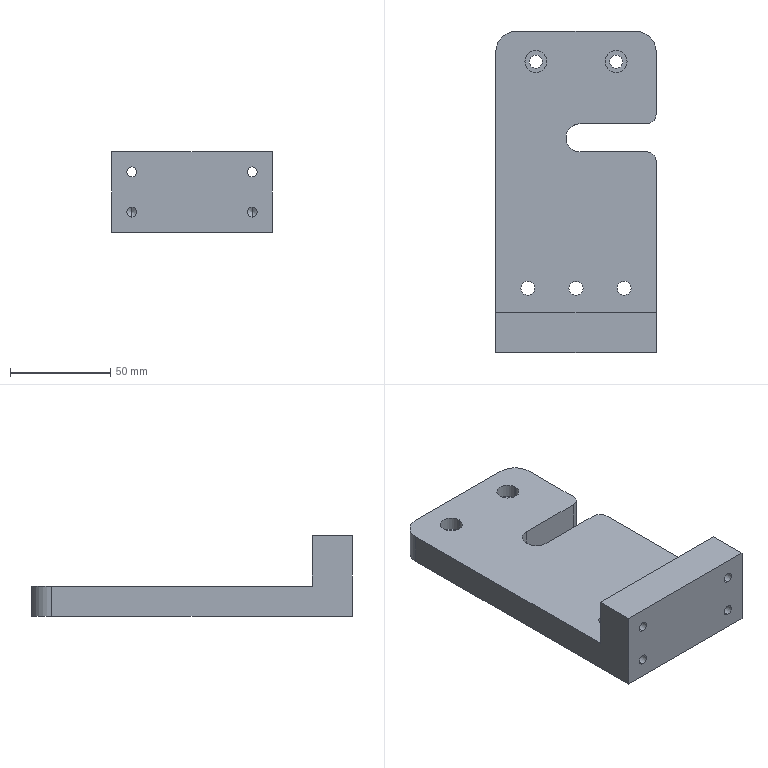Part | SolidWorks | features BaseBody 1 | 1 solid | 44 faces | box 80 x 160 x 40 mm | volume 216767 mm3 | cylinder 27 | plane 13 | cone 4 | commonest cylinder face diameters 5 x8 7 x6 6.6 x4 11 x4 10 x2 20 x2
STEP:
#1=CARTESIAN_POINT('',(-25.5,65.,8.2));
#2=VERTEX_POINT('',#1);
#3=CARTESIAN_POINT('',(-14.5,65.,8.2));
#4=VERTEX_POINT('',#3);
#5=CARTESIAN_POINT('',(-20.,65.,8.2));
#6=DIRECTION('',(0.,0.,1.));
#7=DIRECTION('',(1.,0.,0.));
#8=AXIS2_PLACEMENT_3D('',#5,#6,#7);
#9=CIRCLE('',#8,5.5);
#10=EDGE_CURVE('',#2,#4,#9,.T.);
#11=ORIENTED_EDGE('',*,*,#10,.F.);
#12=CARTESIAN_POINT('',(-25.5,65.,15.));
#13=VERTEX_POINT('',#12);
#14=CARTESIAN_POINT('',(-25.5,65.,15.));
#15=DIRECTION('',(0.,0.,1.));
#16=VECTOR('',#15,1000.);
#17=LINE('',#14,#16);
#18=EDGE_CURVE('',#2,#13,#17,.T.);
#19=ORIENTED_EDGE('',*,*,#18,.T.);
#20=CARTESIAN_POINT('',(-14.5,65.,15.));
#21=VERTEX_POINT('',#20);
#22=CARTESIAN_POINT('',(-20.,65.,15.));
#23=DIRECTION('',(0.,0.,1.));
#24=DIRECTION('',(1.,0.,0.));
#25=AXIS2_PLACEMENT_3D('',#22,#23,#24);
#26=CIRCLE('',#25,5.5);
#27=EDGE_CURVE('',#13,#21,#26,.T.);
#28=ORIENTED_EDGE('',*,*,#27,.T.);
#29=CARTESIAN_POINT('',(-14.5,65.,15.));
#30=DIRECTION('',(0.,0.,1.));
#31=VECTOR('',#30,1000.);
#32=LINE('',#29,#31);
#33=EDGE_CURVE('',#4,#21,#32,.T.);
#34=ORIENTED_EDGE('',*,*,#33,.F.);
#35=EDGE_LOOP('',(#11,#19,#28,#34));
#36=FACE_OUTER_BOUND('',#35,.T.);
#37=CARTESIAN_POINT('',(-20.,65.,15.));
#38=DIRECTION('',(0.,0.,1.));
#39=DIRECTION('',(1.,0.,0.));
#40=AXIS2_PLACEMENT_3D('',#37,#38,#39);
#41=CYLINDRICAL_SURFACE('',#40,5.5);
#42=ADVANCED_FACE('',(#36),#41,.F.);
#43=CARTESIAN_POINT('',(-23.3,65.,0.));
#44=VERTEX_POINT('',#43);
#45=CARTESIAN_POINT('',(-16.7,65.,0.));
#46=VERTEX_POINT('',#45);
#47=CARTESIAN_POINT('',(-20.,65.,0.));
#48=DIRECTION('',(0.,0.,1.));
#49=DIRECTION('',(1.,0.,0.));
#50=AXIS2_PLACEMENT_3D('',#47,#48,#49);
#51=CIRCLE('',#50,3.3);
#52=EDGE_CURVE('',#44,#46,#51,.T.);
#53=ORIENTED_EDGE('',*,*,#52,.F.);
#54=CARTESIAN_POINT('',(-23.3,65.,8.2));
#55=VERTEX_POINT('',#54);
#56=CARTESIAN_POINT('',(-23.3,65.,15.));
#57=DIRECTION('',(0.,0.,1.));
#58=VECTOR('',#57,1000.);
#59=LINE('',#56,#58);
#60=EDGE_CURVE('',#44,#55,#59,.T.);
#61=ORIENTED_EDGE('',*,*,#60,.T.);
#62=CARTESIAN_POINT('',(-16.7,65.,8.2));
#63=VERTEX_POINT('',#62);
#64=CARTESIAN_POINT('',(-20.,65.,8.2));
#65=DIRECTION('',(0.,0.,1.));
#66=DIRECTION('',(1.,0.,0.));
#67=AXIS2_PLACEMENT_3D('',#64,#65,#66);
#68=CIRCLE('',#67,3.3);
#69=EDGE_CURVE('',#55,#63,#68,.T.);
#70=ORIENTED_EDGE('',*,*,#69,.T.);
#71=CARTESIAN_POINT('',(-16.7,65.,15.));
#72=DIRECTION('',(0.,0.,1.));
#73=VECTOR('',#72,1000.);
#74=LINE('',#71,#73);
#75=EDGE_CURVE('',#46,#63,#74,.T.);
#76=ORIENTED_EDGE('',*,*,#75,.F.);
#77=EDGE_LOOP('',(#53,#61,#70,#76));
#78=FACE_OUTER_BOUND('',#77,.T.);
#79=CARTESIAN_POINT('',(-20.,65.,15.));
#80=DIRECTION('',(0.,0.,1.));
#81=DIRECTION('',(1.,0.,0.));
#82=AXIS2_PLACEMENT_3D('',#79,#80,#81);
#83=CYLINDRICAL_SURFACE('',#82,3.3);
#84=ADVANCED_FACE('',(#78),#83,.F.);
#85=CARTESIAN_POINT('',(14.5,65.,8.2));
#86=VERTEX_POINT('',#85);
#87=CARTESIAN_POINT('',(25.5,65.,8.2));
#88=VERTEX_POINT('',#87);
#89=CARTESIAN_POINT('',(20.,65.,8.2));
#90=DIRECTION('',(0.,0.,1.));
#91=DIRECTION('',(1.,0.,0.));
#92=AXIS2_PLACEMENT_3D('',#89,#90,#91);
#93=CIRCLE('',#92,5.5);
#94=EDGE_CURVE('',#86,#88,#93,.T.);
#95=ORIENTED_EDGE('',*,*,#94,.F.);
#96=CARTESIAN_POINT('',(14.5,65.,15.));
#97=VERTEX_POINT('',#96);
#98=CARTESIAN_POINT('',(14.5,65.,15.));
#99=DIRECTION('',(0.,0.,1.));
#100=VECTOR('',#99,1000.);
#101=LINE('',#98,#100);
#102=EDGE_CURVE('',#86,#97,#101,.T.);
#103=ORIENTED_EDGE('',*,*,#102,.T.);
#104=CARTESIAN_POINT('',(25.5,65.,15.));
#105=VERTEX_POINT('',#104);
#106=CARTESIAN_POINT('',(20.,65.,15.));
#107=DIRECTION('',(0.,0.,1.));
#108=DIRECTION('',(1.,0.,0.));
#109=AXIS2_PLACEMENT_3D('',#106,#107,#108);
#110=CIRCLE('',#109,5.5);
#111=EDGE_CURVE('',#97,#105,#110,.T.);
#112=ORIENTED_EDGE('',*,*,#111,.T.);
#113=CARTESIAN_POINT('',(25.5,65.,15.));
#114=DIRECTION('',(0.,0.,1.));
#115=VECTOR('',#114,1000.);
#116=LINE('',#113,#115);
#117=EDGE_CURVE('',#88,#105,#116,.T.);
#118=ORIENTED_EDGE('',*,*,#117,.F.);
#119=EDGE_LOOP('',(#95,#103,#112,#118));
#120=FACE_OUTER_BOUND('',#119,.T.);
#121=CARTESIAN_POINT('',(20.,65.,15.));
#122=DIRECTION('',(0.,0.,1.));
#123=DIRECTION('',(1.,0.,0.));
#124=AXIS2_PLACEMENT_3D('',#121,#122,#123);
#125=CYLINDRICAL_SURFACE('',#124,5.5);
#126=ADVANCED_FACE('',(#120),#125,.F.);
#127=CARTESIAN_POINT('',(16.7,65.,0.));
#128=VERTEX_POINT('',#127);
#129=CARTESIAN_POINT('',(23.3,65.,0.));
#130=VERTEX_POINT('',#129);
#131=CARTESIAN_POINT('',(20.,65.,0.));
#132=DIRECTION('',(0.,0.,1.));
#133=DIRECTION('',(1.,0.,0.));
#134=AXIS2_PLACEMENT_3D('',#131,#132,#133);
#135=CIRCLE('',#134,3.3);
#136=EDGE_CURVE('',#128,#130,#135,.T.);
#137=ORIENTED_EDGE('',*,*,#136,.F.);
#138=CARTESIAN_POINT('',(16.7,65.,8.2));
#139=VERTEX_POINT('',#138);
#140=CARTESIAN_POINT('',(16.7,65.,15.));
#141=DIRECTION('',(0.,0.,1.));
#142=VECTOR('',#141,1000.);
#143=LINE('',#140,#142);
#144=EDGE_CURVE('',#128,#139,#143,.T.);
#145=ORIENTED_EDGE('',*,*,#144,.T.);
#146=CARTESIAN_POINT('',(23.3,65.,8.2));
#147=VERTEX_POINT('',#146);
#148=CARTESIAN_POINT('',(20.,65.,8.2));
#149=DIRECTION('',(0.,0.,1.));
#150=DIRECTION('',(1.,0.,0.));
#151=AXIS2_PLACEMENT_3D('',#148,#149,#150);
#152=CIRCLE('',#151,3.3);
#153=EDGE_CURVE('',#139,#147,#152,.T.);
#154=ORIENTED_EDGE('',*,*,#153,.T.);
#155=CARTESIAN_POINT('',(23.3,65.,15.));
#156=DIRECTION('',(0.,0.,1.));
#157=VECTOR('',#156,1000.);
#158=LINE('',#155,#157);
#159=EDGE_CURVE('',#130,#147,#158,.T.);
#160=ORIENTED_EDGE('',*,*,#159,.F.);
#161=EDGE_LOOP('',(#137,#145,#154,#160));
#162=FACE_OUTER_BOUND('',#161,.T.);
#163=CARTESIAN_POINT('',(20.,65.,15.));
#164=DIRECTION('',(0.,0.,1.));
#165=DIRECTION('',(1.,0.,0.));
#166=AXIS2_PLACEMENT_3D('',#163,#164,#165);
#167=CYLINDRICAL_SURFACE('',#166,3.3);
#168=ADVANCED_FACE('',(#162),#167,.F.);
#169=CARTESIAN_POINT('',(-27.5,-48.,0.));
#170=VERTEX_POINT('',#169);
#171=CARTESIAN_POINT('',(-20.5,-48.,0.));
#172=VERTEX_POINT('',#171);
#173=CARTESIAN_POINT('',(-24.,-48.,0.));
#174=DIRECTION('',(0.,0.,1.));
#175=DIRECTION('',(1.,0.,0.));
#176=AXIS2_PLACEMENT_3D('',#173,#174,#175);
#177=CIRCLE('',#176,3.5);
#178=EDGE_CURVE('',#170,#172,#177,.T.);
#179=ORIENTED_EDGE('',*,*,#178,.F.);
#180=CARTESIAN_POINT('',(-27.5,-48.,15.));
#181=VERTEX_POINT('',#180);
#182=CARTESIAN_POINT('',(-27.5,-48.,15.));
#183=DIRECTION('',(0.,0.,1.));
#184=VECTOR('',#183,1000.);
#185=LINE('',#182,#184);
#186=EDGE_CURVE('',#170,#181,#185,.T.);
#187=ORIENTED_EDGE('',*,*,#186,.T.);
#188=CARTESIAN_POINT('',(-20.5,-48.,15.));
#189=VERTEX_POINT('',#188);
#190=CARTESIAN_POINT('',(-24.,-48.,15.));
#191=DIRECTION('',(0.,0.,1.));
#192=DIRECTION('',(1.,0.,0.));
#193=AXIS2_PLACEMENT_3D('',#190,#191,#192);
#194=CIRCLE('',#193,3.5);
#195=EDGE_CURVE('',#181,#189,#194,.T.);
#196=ORIENTED_EDGE('',*,*,#195,.T.);
#197=CARTESIAN_POINT('',(-20.5,-48.,15.));
#198=DIRECTION('',(0.,0.,1.));
#199=VECTOR('',#198,1000.);
#200=LINE('',#197,#199);
#201=EDGE_CURVE('',#172,#189,#200,.T.);
#202=ORIENTED_EDGE('',*,*,#201,.F.);
#203=EDGE_LOOP('',(#179,#187,#196,#202));
#204=FACE_OUTER_BOUND('',#203,.T.);
#205=CARTESIAN_POINT('',(-24.,-48.,15.));
#206=DIRECTION('',(0.,0.,1.));
#207=DIRECTION('',(1.,0.,0.));
#208=AXIS2_PLACEMENT_3D('',#205,#206,#207);
#209=CYLINDRICAL_SURFACE('',#208,3.5);
#210=ADVANCED_FACE('',(#204),#209,.F.);
#211=CARTESIAN_POINT('',(-3.5,-48.,0.));
#212=VERTEX_POINT('',#211);
#213=CARTESIAN_POINT('',(3.5,-48.,0.));
#214=VERTEX_POINT('',#213);
#215=CARTESIAN_POINT('',(0.,-48.,0.));
#216=DIRECTION('',(0.,0.,1.));
#217=DIRECTION('',(1.,0.,0.));
#218=AXIS2_PLACEMENT_3D('',#215,#216,#217);
#219=CIRCLE('',#218,3.5);
#220=EDGE_CURVE('',#212,#214,#219,.T.);
#221=ORIENTED_EDGE('',*,*,#220,.F.);
#222=CARTESIAN_POINT('',(-3.5,-48.,15.));
#223=VERTEX_POINT('',#222);
#224=CARTESIAN_POINT('',(-3.5,-48.,15.));
#225=DIRECTION('',(0.,0.,1.));
#226=VECTOR('',#225,1000.);
#227=LINE('',#224,#226);
#228=EDGE_CURVE('',#212,#223,#227,.T.);
#229=ORIENTED_EDGE('',*,*,#228,.T.);
#230=CARTESIAN_POINT('',(3.5,-48.,15.));
#231=VERTEX_POINT('',#230);
#232=CARTESIAN_POINT('',(0.,-48.,15.));
#233=DIRECTION('',(0.,0.,1.));
#234=DIRECTION('',(1.,0.,0.));
#235=AXIS2_PLACEMENT_3D('',#232,#233,#234);
#236=CIRCLE('',#235,3.5);
#237=EDGE_CURVE('',#223,#231,#236,.T.);
#238=ORIENTED_EDGE('',*,*,#237,.T.);
#239=CARTESIAN_POINT('',(3.5,-48.,15.));
#240=DIRECTION('',(0.,0.,1.));
#241=VECTOR('',#240,1000.);
#242=LINE('',#239,#241);
#243=EDGE_CURVE('',#214,#231,#242,.T.);
#244=ORIENTED_EDGE('',*,*,#243,.F.);
#245=EDGE_LOOP('',(#221,#229,#238,#244));
#246=FACE_OUTER_BOUND('',#245,.T.);
#247=CARTESIAN_POINT('',(0.,-48.,15.));
#248=DIRECTION('',(0.,0.,1.));
#249=DIRECTION('',(1.,0.,0.));
#250=AXIS2_PLACEMENT_3D('',#247,#248,#249);
#251=CYLINDRICAL_SURFACE('',#250,3.5);
#252=ADVANCED_FACE('',(#246),#251,.F.);
#253=CARTESIAN_POINT('',(20.5,-48.,0.));
#254=VERTEX_POINT('',#253);
#255=CARTESIAN_POINT('',(27.5,-48.,0.));
#256=VERTEX_POINT('',#255);
#257=CARTESIAN_POINT('',(24.,-48.,0.));
#258=DIRECTION('',(0.,0.,1.));
#259=DIRECTION('',(1.,0.,0.));
#260=AXIS2_PLACEMENT_3D('',#257,#258,#259);
#261=CIRCLE('',#260,3.5);
#262=EDGE_CURVE('',#254,#256,#261,.T.);
#263=ORIENTED_EDGE('',*,*,#262,.F.);
#264=CARTESIAN_POINT('',(20.5,-48.,15.));
#265=VERTEX_POINT('',#264);
#266=CARTESIAN_POINT('',(20.5,-48.,15.));
#267=DIRECTION('',(0.,0.,1.));
#268=VECTOR('',#267,1000.);
#269=LINE('',#266,#268);
#270=EDGE_CURVE('',#254,#265,#269,.T.);
#271=ORIENTED_EDGE('',*,*,#270,.T.);
#272=CARTESIAN_POINT('',(27.5,-48.,15.));
#273=VERTEX_POINT('',#272);
#274=CARTESIAN_POINT('',(24.,-48.,15.));
#275=DIRECTION('',(0.,0.,1.));
#276=DIRECTION('',(1.,0.,0.));
#277=AXIS2_PLACEMENT_3D('',#274,#275,#276);
#278=CIRCLE('',#277,3.5);
#279=EDGE_CURVE('',#265,#273,#278,.T.);
#280=ORIENTED_EDGE('',*,*,#279,.T.);
#281=CARTESIAN_POINT('',(27.5,-48.,15.));
#282=DIRECTION('',(0.,0.,1.));
#283=VECTOR('',#282,1000.);
#284=LINE('',#281,#283);
#285=EDGE_CURVE('',#256,#273,#284,.T.);
#286=ORIENTED_EDGE('',*,*,#285,.F.);
#287=EDGE_LOOP('',(#263,#271,#280,#286));
#288=FACE_OUTER_BOUND('',#287,.T.);
#289=CARTESIAN_POINT('',(24.,-48.,15.));
#290=DIRECTION('',(0.,0.,1.));
#291=DIRECTION('',(1.,0.,0.));
#292=AXIS2_PLACEMENT_3D('',#289,#290,#291);
#293=CYLINDRICAL_SURFACE('',#292,3.5);
#294=ADVANCED_FACE('',(#288),#293,.F.);
#295=CARTESIAN_POINT('',(30.,-60.,32.5));
#296=VERTEX_POINT('',#295);
#297=CARTESIAN_POINT('',(30.,-60.,27.5));
#298=VERTEX_POINT('',#297);
#299=CARTESIAN_POINT('',(30.,-60.,30.));
#300=DIRECTION('',(0.,-1.,0.));
#301=DIRECTION('',(0.,0.,-1.));
#302=AXIS2_PLACEMENT_3D('',#299,#300,#301);
#303=CIRCLE('',#302,2.5);
#304=EDGE_CURVE('',#296,#298,#303,.T.);
#305=ORIENTED_EDGE('',*,*,#304,.F.);
#306=CARTESIAN_POINT('',(30.,-80.,32.5));
#307=VERTEX_POINT('',#306);
#308=CARTESIAN_POINT('',(30.,-80.,32.5));
#309=DIRECTION('',(0.,-1.,0.));
#310=VECTOR('',#309,1000.);
#311=LINE('',#308,#310);
#312=EDGE_CURVE('',#296,#307,#311,.T.);
#313=ORIENTED_EDGE('',*,*,#312,.T.);
#314=CARTESIAN_POINT('',(30.,-80.,27.5));
#315=VERTEX_POINT('',#314);
#316=CARTESIAN_POINT('',(30.,-80.,30.));
#317=DIRECTION('',(0.,-1.,0.));
#318=DIRECTION('',(0.,0.,-1.));
#319=AXIS2_PLACEMENT_3D('',#316,#317,#318);
#320=CIRCLE('',#319,2.5);
#321=EDGE_CURVE('',#307,#315,#320,.T.);
#322=ORIENTED_EDGE('',*,*,#321,.T.);
#323=CARTESIAN_POINT('',(30.,-80.,27.5));
#324=DIRECTION('',(0.,-1.,0.));
#325=VECTOR('',#324,1000.);
#326=LINE('',#323,#325);
#327=EDGE_CURVE('',#298,#315,#326,.T.);
#328=ORIENTED_EDGE('',*,*,#327,.F.);
#329=EDGE_LOOP('',(#305,#313,#322,#328));
#330=FACE_OUTER_BOUND('',#329,.T.);
#331=CARTESIAN_POINT('',(30.,-80.,30.));
#332=DIRECTION('',(0.,-1.,0.));
#333=DIRECTION('',(0.,0.,-1.));
#334=AXIS2_PLACEMENT_3D('',#331,#332,#333);
#335=CYLINDRICAL_SURFACE('',#334,2.5);
#336=ADVANCED_FACE('',(#330),#335,.F.);
#337=CARTESIAN_POINT('',(30.,-57.,12.5));
#338=VERTEX_POINT('',#337);
#339=CARTESIAN_POINT('',(30.,-57.,7.5));
#340=VERTEX_POINT('',#339);
#341=CARTESIAN_POINT('',(30.,-57.,10.));
#342=DIRECTION('',(0.,-1.,0.));
#343=DIRECTION('',(0.,0.,-1.));
#344=AXIS2_PLACEMENT_3D('',#341,#342,#343);
#345=CIRCLE('',#344,2.5);
#346=EDGE_CURVE('',#338,#340,#345,.T.);
#347=ORIENTED_EDGE('',*,*,#346,.F.);
#348=CARTESIAN_POINT('',(30.,-80.,12.5));
#349=VERTEX_POINT('',#348);
#350=CARTESIAN_POINT('',(30.,-80.,12.5));
#351=DIRECTION('',(0.,-1.,0.));
#352=VECTOR('',#351,1000.);
#353=LINE('',#350,#352);
#354=EDGE_CURVE('',#338,#349,#353,.T.);
#355=ORIENTED_EDGE('',*,*,#354,.T.);
#356=CARTESIAN_POINT('',(30.,-80.,7.5));
#357=VERTEX_POINT('',#356);
#358=CARTESIAN_POINT('',(30.,-80.,10.));
#359=DIRECTION('',(0.,-1.,0.));
#360=DIRECTION('',(0.,0.,-1.));
#361=AXIS2_PLACEMENT_3D('',#358,#359,#360);
#362=CIRCLE('',#361,2.5);
#363=EDGE_CURVE('',#349,#357,#362,.T.);
#364=ORIENTED_EDGE('',*,*,#363,.T.);
#365=CARTESIAN_POINT('',(30.,-80.,7.5));
#366=DIRECTION('',(0.,-1.,0.));
#367=VECTOR('',#366,1000.);
#368=LINE('',#365,#367);
#369=EDGE_CURVE('',#340,#357,#368,.T.);
#370=ORIENTED_EDGE('',*,*,#369,.F.);
#371=EDGE_LOOP('',(#347,#355,#364,#370));
#372=FACE_OUTER_BOUND('',#371,.T.);
#373=CARTESIAN_POINT('',(30.,-80.,10.));
#374=DIRECTION('',(0.,-1.,0.));
#375=DIRECTION('',(0.,0.,-1.));
#376=AXIS2_PLACEMENT_3D('',#373,#374,#375);
#377=CYLINDRICAL_SURFACE('',#376,2.5);
#378=ADVANCED_FACE('',(#372),#377,.F.);
#379=CARTESIAN_POINT('',(30.,-55.498,10.));
#380=VERTEX_POINT('',#379);
#381=CARTESIAN_POINT('',(30.,-57.,7.5));
#382=DIRECTION('',(0.,-0.515,-0.8572));
#383=VECTOR('',#382,1000.);
#384=LINE('',#381,#383);
#385=EDGE_CURVE('',#380,#340,#384,.T.);
#386=ORIENTED_EDGE('',*,*,#385,.F.);
#387=CARTESIAN_POINT('',(30.,-57.,12.5));
#388=DIRECTION('',(0.,-0.515,0.8572));
#389=VECTOR('',#388,1000.);
#390=LINE('',#387,#389);
#391=EDGE_CURVE('',#380,#338,#390,.T.);
#392=ORIENTED_EDGE('',*,*,#391,.T.);
#393=ORIENTED_EDGE('',*,*,#346,.T.);
#394=EDGE_LOOP('',(#386,#392,#393));
#395=FACE_OUTER_BOUND('',#394,.T.);
#396=CARTESIAN_POINT('',(30.,-57.,10.));
#397=DIRECTION('',(0.,-1.,0.));
#398=DIRECTION('',(0.,0.,-1.));
#399=AXIS2_PLACEMENT_3D('',#396,#397,#398);
#400=CONICAL_SURFACE('',#399,2.5,1.03);
#401=ADVANCED_FACE('',(#395),#400,.F.);
#402=CARTESIAN_POINT('',(-30.,-57.,12.5));
#403=VERTEX_POINT('',#402);
#404=CARTESIAN_POINT('',(-30.,-57.,7.5));
#405=VERTEX_POINT('',#404);
#406=CARTESIAN_POINT('',(-30.,-57.,10.));
#407=DIRECTION('',(0.,-1.,0.));
#408=DIRECTION('',(0.,0.,-1.));
#409=AXIS2_PLACEMENT_3D('',#406,#407,#408);
#410=CIRCLE('',#409,2.5);
#411=EDGE_CURVE('',#403,#405,#410,.T.);
#412=ORIENTED_EDGE('',*,*,#411,.F.);
#413=CARTESIAN_POINT('',(-30.,-80.,12.5));
#414=VERTEX_POINT('',#413);
#415=CARTESIAN_POINT('',(-30.,-80.,12.5));
#416=DIRECTION('',(0.,-1.,0.));
#417=VECTOR('',#416,1000.);
#418=LINE('',#415,#417);
#419=EDGE_CURVE('',#403,#414,#418,.T.);
#420=ORIENTED_EDGE('',*,*,#419,.T.);
#421=CARTESIAN_POINT('',(-30.,-80.,7.5));
#422=VERTEX_POINT('',#421);
#423=CARTESIAN_POINT('',(-30.,-80.,10.));
#424=DIRECTION('',(0.,-1.,0.));
#425=DIRECTION('',(0.,0.,-1.));
#426=AXIS2_PLACEMENT_3D('',#423,#424,#425);
#427=CIRCLE('',#426,2.5);
#428=EDGE_CURVE('',#414,#422,#427,.T.);
#429=ORIENTED_EDGE('',*,*,#428,.T.);
#430=CARTESIAN_POINT('',(-30.,-80.,7.5));
#431=DIRECTION('',(0.,-1.,0.));
#432=VECTOR('',#431,1000.);
#433=LINE('',#430,#432);
#434=EDGE_CURVE('',#405,#422,#433,.T.);
#435=ORIENTED_EDGE('',*,*,#434,.F.);
#436=EDGE_LOOP('',(#412,#420,#429,#435));
#437=FACE_OUTER_BOUND('',#436,.T.);
#438=CARTESIAN_POINT('',(-30.,-80.,10.));
#439=DIRECTION('',(0.,-1.,0.));
#440=DIRECTION('',(0.,0.,-1.));
#441=AXIS2_PLACEMENT_3D('',#438,#439,#440);
#442=CYLINDRICAL_SURFACE('',#441,2.5);
#443=ADVANCED_FACE('',(#437),#442,.F.);
#444=CARTESIAN_POINT('',(-30.,-55.498,10.));
#445=VERTEX_POINT('',#444);
#446=CARTESIAN_POINT('',(-30.,-57.,7.5));
#447=DIRECTION('',(0.,-0.515,-0.8572));
#448=VECTOR('',#447,1000.);
#449=LINE('',#446,#448);
#450=EDGE_CURVE('',#445,#405,#449,.T.);
#451=ORIENTED_EDGE('',*,*,#450,.F.);
#452=CARTESIAN_POINT('',(-30.,-57.,12.5));
#453=DIRECTION('',(0.,-0.515,0.8572));
#454=VECTOR('',#453,1000.);
#455=LINE('',#452,#454);
#456=EDGE_CURVE('',#445,#403,#455,.T.);
#457=ORIENTED_EDGE('',*,*,#456,.T.);
#458=ORIENTED_EDGE('',*,*,#411,.T.);
#459=EDGE_LOOP('',(#451,#457,#458));
#460=FACE_OUTER_BOUND('',#459,.T.);
#461=CARTESIAN_POINT('',(-30.,-57.,10.));
#462=DIRECTION('',(0.,-1.,0.));
#463=DIRECTION('',(0.,0.,-1.));
#464=AXIS2_PLACEMENT_3D('',#461,#462,#463);
#465=CONICAL_SURFACE('',#464,2.5,1.03);
#466=ADVANCED_FACE('',(#460),#465,.F.);
#467=CARTESIAN_POINT('',(-30.,-60.,32.5));
#468=VERTEX_POINT('',#467);
#469=CARTESIAN_POINT('',(-30.,-60.,27.5));
#470=VERTEX_POINT('',#469);
#471=CARTESIAN_POINT('',(-30.,-60.,30.));
#472=DIRECTION('',(0.,-1.,0.));
#473=DIRECTION('',(0.,0.,-1.));
#474=AXIS2_PLACEMENT_3D('',#471,#472,#473);
#475=CIRCLE('',#474,2.5);
#476=EDGE_CURVE('',#468,#470,#475,.T.);
#477=ORIENTED_EDGE('',*,*,#476,.F.);
#478=CARTESIAN_POINT('',(-30.,-80.,32.5));
#479=VERTEX_POINT('',#478);
#480=CARTESIAN_POINT('',(-30.,-80.,32.5));
#481=DIRECTION('',(0.,-1.,0.));
#482=VECTOR('',#481,1000.);
#483=LINE('',#480,#482);
#484=EDGE_CURVE('',#468,#479,#483,.T.);
#485=ORIENTED_EDGE('',*,*,#484,.T.);
#486=CARTESIAN_POINT('',(-30.,-80.,27.5));
#487=VERTEX_POINT('',#486);
#488=CARTESIAN_POINT('',(-30.,-80.,30.));
#489=DIRECTION('',(0.,-1.,0.));
#490=DIRECTION('',(0.,0.,-1.));
#491=AXIS2_PLACEMENT_3D('',#488,#489,#490);
#492=CIRCLE('',#491,2.5);
#493=EDGE_CURVE('',#479,#487,#492,.T.);
#494=ORIENTED_EDGE('',*,*,#493,.T.);
#495=CARTESIAN_POINT('',(-30.,-80.,27.5));
#496=DIRECTION('',(0.,-1.,0.));
#497=VECTOR('',#496,1000.);
#498=LINE('',#495,#497);
#499=EDGE_CURVE('',#470,#487,#498,.T.);
#500=ORIENTED_EDGE('',*,*,#499,.F.);
#501=EDGE_LOOP('',(#477,#485,#494,#500));
#502=FACE_OUTER_BOUND('',#501,.T.);
#503=CARTESIAN_POINT('',(-30.,-80.,30.));
#504=DIRECTION('',(0.,-1.,0.));
#505=DIRECTION('',(0.,0.,-1.));
#506=AXIS2_PLACEMENT_3D('',#503,#504,#505);
#507=CYLINDRICAL_SURFACE('',#506,2.5);
#508=ADVANCED_FACE('',(#502),#507,.F.);
#509=CARTESIAN_POINT('',(40.,39.,0.));
#510=VERTEX_POINT('',#509);
#511=CARTESIAN_POINT('',(35.,34.,0.));
#512=VERTEX_POINT('',#511);
#513=CARTESIAN_POINT('',(35.,39.,0.));
#514=DIRECTION('',(0.,0.,-1.));
#515=DIRECTION('',(1.,0.,0.));
#516=AXIS2_PLACEMENT_3D('',#513,#514,#515);
#517=CIRCLE('',#516,5.);
#518=EDGE_CURVE('',#510,#512,#517,.T.);
#519=ORIENTED_EDGE('',*,*,#518,.F.);
#520=CARTESIAN_POINT('',(40.,39.,15.));
#521=VERTEX_POINT('',#520);
#522=CARTESIAN_POINT('',(40.,39.,40.));
#523=DIRECTION('',(0.,0.,-1.));
#524=VECTOR('',#523,1000.);
#525=LINE('',#522,#524);
#526=EDGE_CURVE('',#521,#510,#525,.T.);
#527=ORIENTED_EDGE('',*,*,#526,.F.);
#528=CARTESIAN_POINT('',(35.,34.,15.));
#529=VERTEX_POINT('',#528);
#530=CARTESIAN_POINT('',(35.,39.,15.));
#531=DIRECTION('',(0.,0.,1.));
#532=DIRECTION('',(-1.,0.,0.));
#533=AXIS2_PLACEMENT_3D('',#530,#531,#532);
#534=CIRCLE('',#533,5.);
#535=EDGE_CURVE('',#529,#521,#534,.T.);
#536=ORIENTED_EDGE('',*,*,#535,.F.);
#537=CARTESIAN_POINT('',(35.,34.,26.866));
#538=DIRECTION('',(0.,0.,1.));
#539=VECTOR('',#538,1000.);
#540=LINE('',#537,#539);
#541=EDGE_CURVE('',#512,#529,#540,.T.);
#542=ORIENTED_EDGE('',*,*,#541,.F.);
#543=EDGE_LOOP('',(#519,#527,#536,#542));
#544=FACE_OUTER_BOUND('',#543,.T.);
#545=CARTESIAN_POINT('',(35.,39.,26.866));
#546=DIRECTION('',(0.,0.,1.));
#547=DIRECTION('',(1.,0.,0.));
#548=AXIS2_PLACEMENT_3D('',#545,#546,#547);
#549=CYLINDRICAL_SURFACE('',#548,5.);
#550=ADVANCED_FACE('',(#544),#549,.T.);
#551=CARTESIAN_POINT('',(40.,15.,15.));
#552=VERTEX_POINT('',#551);
#553=CARTESIAN_POINT('',(35.,20.,15.));
#554=VERTEX_POINT('',#553);
#555=CARTESIAN_POINT('',(35.,15.,15.));
#556=DIRECTION('',(0.,0.,1.));
#557=DIRECTION('',(-1.,0.,0.));
#558=AXIS2_PLACEMENT_3D('',#555,#556,#557);
#559=CIRCLE('',#558,5.);
#560=EDGE_CURVE('',#552,#554,#559,.T.);
#561=ORIENTED_EDGE('',*,*,#560,.F.);
#562=CARTESIAN_POINT('',(40.,15.,0.));
#563=VERTEX_POINT('',#562);
#564=CARTESIAN_POINT('',(40.,15.,40.));
#565=DIRECTION('',(0.,0.,1.));
#566=VECTOR('',#565,1000.);
#567=LINE('',#564,#566);
#568=EDGE_CURVE('',#563,#552,#567,.T.);
#569=ORIENTED_EDGE('',*,*,#568,.F.);
#570=CARTESIAN_POINT('',(35.,20.,0.));
#571=VERTEX_POINT('',#570);
#572=CARTESIAN_POINT('',(35.,15.,0.));
#573=DIRECTION('',(0.,0.,-1.));
#574=DIRECTION('',(1.,0.,0.));
#575=AXIS2_PLACEMENT_3D('',#572,#573,#574);
#576=CIRCLE('',#575,5.);
#577=EDGE_CURVE('',#571,#563,#576,.T.);
#578=ORIENTED_EDGE('',*,*,#577,.F.);
#579=CARTESIAN_POINT('',(35.,20.,26.866));
#580=DIRECTION('',(0.,0.,-1.));
#581=VECTOR('',#580,1000.);
#582=LINE('',#579,#581);
#583=EDGE_CURVE('',#554,#571,#582,.T.);
#584=ORIENTED_EDGE('',*,*,#583,.F.);
#585=EDGE_LOOP('',(#561,#569,#578,#584));
#586=FACE_OUTER_BOUND('',#585,.T.);
#587=CARTESIAN_POINT('',(35.,15.,26.866));
#588=DIRECTION('',(0.,0.,-1.));
#589=DIRECTION('',(-1.,0.,0.));
#590=AXIS2_PLACEMENT_3D('',#587,#588,#589);
#591=CYLINDRICAL_SURFACE('',#590,5.);
#592=ADVANCED_FACE('',(#586),#591,.T.);
#593=CARTESIAN_POINT('',(-20.,65.,8.2));
#594=DIRECTION('',(0.,0.,1.));
#595=DIRECTION('',(1.,0.,0.));
#596=AXIS2_PLACEMENT_3D('',#593,#594,#595);
#597=CIRCLE('',#596,3.3);
#598=EDGE_CURVE('',#63,#55,#597,.T.);
#599=ORIENTED_EDGE('',*,*,#598,.F.);
#600=ORIENTED_EDGE('',*,*,#69,.F.);
#601=EDGE_LOOP('',(#599,#600));
#602=FACE_BOUND('',#601,.T.);
#603=CARTESIAN_POINT('',(-20.,65.,8.2));
#604=DIRECTION('',(0.,0.,1.));
#605=DIRECTION('',(1.,0.,0.));
#606=AXIS2_PLACEMENT_3D('',#603,#604,#605);
#607=CIRCLE('',#606,5.5);
#608=EDGE_CURVE('',#4,#2,#607,.T.);
#609=ORIENTED_EDGE('',*,*,#608,.T.);
#610=ORIENTED_EDGE('',*,*,#10,.T.);
#611=EDGE_LOOP('',(#609,#610));
#612=FACE_OUTER_BOUND('',#611,.T.);
#613=CARTESIAN_POINT('',(-16.7,65.,8.2));
#614=DIRECTION('',(0.,0.,-1.));
#615=DIRECTION('',(0.,-1.,0.));
#616=AXIS2_PLACEMENT_3D('',#613,#614,#615);
#617=PLANE('',#616);
#618=ADVANCED_FACE('',(#602,#612),#617,.F.);
#619=CARTESIAN_POINT('',(20.,65.,8.2));
#620=DIRECTION('',(0.,0.,1.));
#621=DIRECTION('',(1.,0.,0.));
#622=AXIS2_PLACEMENT_3D('',#619,#620,#621);
#623=CIRCLE('',#622,3.3);
#624=EDGE_CURVE('',#147,#139,#623,.T.);
#625=ORIENTED_EDGE('',*,*,#624,.F.);
#626=ORIENTED_EDGE('',*,*,#153,.F.);
#627=EDGE_LOOP('',(#625,#626));
#628=FACE_BOUND('',#627,.T.);
#629=CARTESIAN_POINT('',(20.,65.,8.2));
#630=DIRECTION('',(0.,0.,1.));
#631=DIRECTION('',(1.,0.,0.));
#632=AXIS2_PLACEMENT_3D('',#629,#630,#631);
#633=CIRCLE('',#632,5.5);
#634=EDGE_CURVE('',#88,#86,#633,.T.);
#635=ORIENTED_EDGE('',*,*,#634,.T.);
#636=ORIENTED_EDGE('',*,*,#94,.T.);
#637=EDGE_LOOP('',(#635,#636));
#638=FACE_OUTER_BOUND('',#637,.T.);
#639=CARTESIAN_POINT('',(23.3,65.,8.2));
#640=DIRECTION('',(0.,0.,-1.));
#641=DIRECTION('',(0.,-1.,0.));
#642=AXIS2_PLACEMENT_3D('',#639,#640,#641);
#643=PLANE('',#642);
#644=ADVANCED_FACE('',(#628,#638),#643,.F.);
#645=CARTESIAN_POINT('',(2.,20.,0.));
#646=VERTEX_POINT('',#645);
#647=CARTESIAN_POINT('',(2.,20.,15.));
#648=VERTEX_POINT('',#647);
#649=CARTESIAN_POINT('',(2.,20.,15.));
#650=DIRECTION('',(0.,0.,1.));
#651=VECTOR('',#650,1000.);
#652=LINE('',#649,#651);
#653=EDGE_CURVE('',#646,#648,#652,.T.);
#654=ORIENTED_EDGE('',*,*,#653,.F.);
#655=CARTESIAN_POINT('',(2.,34.,0.));
#656=VERTEX_POINT('',#655);
#657=CARTESIAN_POINT('',(2.,27.,0.));
#658=DIRECTION('',(0.,0.,1.));
#659=DIRECTION('',(1.,0.,0.));
#660=AXIS2_PLACEMENT_3D('',#657,#658,#659);
#661=CIRCLE('',#660,7.);
#662=EDGE_CURVE('',#656,#646,#661,.T.);
#663=ORIENTED_EDGE('',*,*,#662,.F.);
#664=CARTESIAN_POINT('',(2.,34.,15.));
#665=VERTEX_POINT('',#664);
#666=CARTESIAN_POINT('',(2.,34.,0.));
#667=DIRECTION('',(0.,0.,-1.));
#668=VECTOR('',#667,1000.);
#669=LINE('',#666,#668);
#670=EDGE_CURVE('',#665,#656,#669,.T.);
#671=ORIENTED_EDGE('',*,*,#670,.F.);
#672=CARTESIAN_POINT('',(2.,27.,15.));
#673=DIRECTION('',(0.,0.,-1.));
#674=DIRECTION('',(-1.,0.,0.));
#675=AXIS2_PLACEMENT_3D('',#672,#673,#674);
#676=CIRCLE('',#675,7.);
#677=EDGE_CURVE('',#648,#665,#676,.T.);
#678=ORIENTED_EDGE('',*,*,#677,.F.);
#679=EDGE_LOOP('',(#654,#663,#671,#678));
#680=FACE_OUTER_BOUND('',#679,.T.);
#681=CARTESIAN_POINT('',(2.,27.,0.));
#682=DIRECTION('',(0.,0.,1.));
#683=DIRECTION('',(1.,0.,0.));
#684=AXIS2_PLACEMENT_3D('',#681,#682,#683);
#685=CYLINDRICAL_SURFACE('',#684,7.);
#686=ADVANCED_FACE('',(#680),#685,.F.);
#687=CARTESIAN_POINT('',(0.,34.,0.));
#688=DIRECTION('',(-1.,0.,0.));
#689=VECTOR('',#688,1000.);
#690=LINE('',#687,#689);
#691=EDGE_CURVE('',#512,#656,#690,.T.);
#692=ORIENTED_EDGE('',*,*,#691,.F.);
#693=ORIENTED_EDGE('',*,*,#541,.T.);
#694=CARTESIAN_POINT('',(-40.,34.,15.));
#695=DIRECTION('',(1.,0.,0.));
#696=VECTOR('',#695,1000.);
#697=LINE('',#694,#696);
#698=EDGE_CURVE('',#665,#529,#697,.T.);
#699=ORIENTED_EDGE('',*,*,#698,.F.);
#700=ORIENTED_EDGE('',*,*,#670,.T.);
#701=EDGE_LOOP('',(#692,#693,#699,#700));
#702=FACE_OUTER_BOUND('',#701,.T.);
#703=CARTESIAN_POINT('',(-5.,34.,26.866));
#704=DIRECTION('',(0.,1.,0.));
#705=DIRECTION('',(1.,0.,0.));
#706=AXIS2_PLACEMENT_3D('',#703,#704,#705);
#707=PLANE('',#706);
#708=ADVANCED_FACE('',(#702),#707,.F.);
#709=CARTESIAN_POINT('',(-40.,20.,15.));
#710=DIRECTION('',(-1.,0.,0.));
#711=VECTOR('',#710,1000.);
#712=LINE('',#709,#711);
#713=EDGE_CURVE('',#554,#648,#712,.T.);
#714=ORIENTED_EDGE('',*,*,#713,.F.);
#715=ORIENTED_EDGE('',*,*,#583,.T.);
#716=CARTESIAN_POINT('',(0.,20.,0.));
#717=DIRECTION('',(1.,0.,0.));
#718=VECTOR('',#717,1000.);
#719=LINE('',#716,#718);
#720=EDGE_CURVE('',#646,#571,#719,.T.);
#721=ORIENTED_EDGE('',*,*,#720,.F.);
#722=ORIENTED_EDGE('',*,*,#653,.T.);
#723=EDGE_LOOP('',(#714,#715,#721,#722));
#724=FACE_OUTER_BOUND('',#723,.T.);
#725=CARTESIAN_POINT('',(-5.,20.,26.866));
#726=DIRECTION('',(0.,-1.,0.));
#727=DIRECTION('',(0.,0.,-1.));
#728=AXIS2_PLACEMENT_3D('',#725,#726,#727);
#729=PLANE('',#728);
#730=ADVANCED_FACE('',(#724),#729,.F.);
#731=CARTESIAN_POINT('',(40.,70.,15.));
#732=VERTEX_POINT('',#731);
#733=CARTESIAN_POINT('',(30.,80.,15.));
#734=VERTEX_POINT('',#733);
#735=CARTESIAN_POINT('',(30.,70.,15.));
#736=DIRECTION('',(0.,0.,1.));
#737=DIRECTION('',(-1.,0.,0.));
#738=AXIS2_PLACEMENT_3D('',#735,#736,#737);
#739=CIRCLE('',#738,10.);
#740=EDGE_CURVE('',#732,#734,#739,.T.);
#741=ORIENTED_EDGE('',*,*,#740,.F.);
#742=CARTESIAN_POINT('',(40.,70.,0.));
#743=VERTEX_POINT('',#742);
#744=CARTESIAN_POINT('',(40.,70.,40.));
#745=DIRECTION('',(0.,0.,1.));
#746=VECTOR('',#745,1000.);
#747=LINE('',#744,#746);
#748=EDGE_CURVE('',#743,#732,#747,.T.);
#749=ORIENTED_EDGE('',*,*,#748,.F.);
#750=CARTESIAN_POINT('',(30.,80.,0.));
#751=VERTEX_POINT('',#750);
#752=CARTESIAN_POINT('',(30.,70.,0.));
#753=DIRECTION('',(0.,0.,-1.));
#754=DIRECTION('',(1.,0.,0.));
#755=AXIS2_PLACEMENT_3D('',#752,#753,#754);
#756=CIRCLE('',#755,10.);
#757=EDGE_CURVE('',#751,#743,#756,.T.);
#758=ORIENTED_EDGE('',*,*,#757,.F.);
#759=CARTESIAN_POINT('',(30.,80.,40.));
#760=DIRECTION('',(0.,0.,-1.));
#761=VECTOR('',#760,1000.);
#762=LINE('',#759,#761);
#763=EDGE_CURVE('',#734,#751,#762,.T.);
#764=ORIENTED_EDGE('',*,*,#763,.F.);
#765=EDGE_LOOP('',(#741,#749,#758,#764));
#766=FACE_OUTER_BOUND('',#765,.T.);
#767=CARTESIAN_POINT('',(30.,70.,40.));
#768=DIRECTION('',(0.,0.,-1.));
#769=DIRECTION('',(-1.,0.,0.));
#770=AXIS2_PLACEMENT_3D('',#767,#768,#769);
#771=CYLINDRICAL_SURFACE('',#770,10.);
#772=ADVANCED_FACE('',(#766),#771,.T.);
#773=CARTESIAN_POINT('',(-30.,80.,15.));
#774=VERTEX_POINT('',#773);
#775=CARTESIAN_POINT('',(-40.,70.,15.));
#776=VERTEX_POINT('',#775);
#777=CARTESIAN_POINT('',(-30.,70.,15.));
#778=DIRECTION('',(0.,0.,1.));
#779=DIRECTION('',(-1.,0.,0.));
#780=AXIS2_PLACEMENT_3D('',#777,#778,#779);
#781=CIRCLE('',#780,10.);
#782=EDGE_CURVE('',#774,#776,#781,.T.);
#783=ORIENTED_EDGE('',*,*,#782,.F.);
#784=CARTESIAN_POINT('',(-30.,80.,0.));
#785=VERTEX_POINT('',#784);
#786=CARTESIAN_POINT('',(-30.,80.,40.));
#787=DIRECTION('',(0.,0.,1.));
#788=VECTOR('',#787,1000.);
#789=LINE('',#786,#788);
#790=EDGE_CURVE('',#785,#774,#789,.T.);
#791=ORIENTED_EDGE('',*,*,#790,.F.);
#792=CARTESIAN_POINT('',(-40.,70.,0.));
#793=VERTEX_POINT('',#792);
#794=CARTESIAN_POINT('',(-30.,70.,0.));
#795=DIRECTION('',(0.,0.,-1.));
#796=DIRECTION('',(1.,0.,0.));
#797=AXIS2_PLACEMENT_3D('',#794,#795,#796);
#798=CIRCLE('',#797,10.);
#799=EDGE_CURVE('',#793,#785,#798,.T.);
#800=ORIENTED_EDGE('',*,*,#799,.F.);
#801=CARTESIAN_POINT('',(-40.,70.,40.));
#802=DIRECTION('',(0.,0.,-1.));
#803=VECTOR('',#802,1000.);
#804=LINE('',#801,#803);
#805=EDGE_CURVE('',#776,#793,#804,.T.);
#806=ORIENTED_EDGE('',*,*,#805,.F.);
#807=EDGE_LOOP('',(#783,#791,#800,#806));
#808=FACE_OUTER_BOUND('',#807,.T.);
#809=CARTESIAN_POINT('',(-30.,70.,40.));
#810=DIRECTION('',(0.,0.,-1.));
#811=DIRECTION('',(-1.,0.,0.));
#812=AXIS2_PLACEMENT_3D('',#809,#810,#811);
#813=CYLINDRICAL_SURFACE('',#812,10.);
#814=ADVANCED_FACE('',(#808),#813,.T.);
#815=CARTESIAN_POINT('',(-30.,-60.,30.));
#816=DIRECTION('',(0.,-1.,0.));
#817=DIRECTION('',(0.,0.,-1.));
#818=AXIS2_PLACEMENT_3D('',#815,#816,#817);
#819=CIRCLE('',#818,2.5);
#820=EDGE_CURVE('',#470,#468,#819,.T.);
#821=ORIENTED_EDGE('',*,*,#820,.T.);
#822=ORIENTED_EDGE('',*,*,#476,.T.);
#823=EDGE_LOOP('',(#821,#822));
#824=FACE_BOUND('',#823,.T.);
#825=CARTESIAN_POINT('',(30.,-60.,30.));
#826=DIRECTION('',(0.,-1.,0.));
#827=DIRECTION('',(0.,0.,-1.));
#828=AXIS2_PLACEMENT_3D('',#825,#826,#827);
#829=CIRCLE('',#828,2.5);
#830=EDGE_CURVE('',#298,#296,#829,.T.);
#831=ORIENTED_EDGE('',*,*,#830,.T.);
#832=ORIENTED_EDGE('',*,*,#304,.T.);
#833=EDGE_LOOP('',(#831,#832));
#834=FACE_BOUND('',#833,.T.);
#835=CARTESIAN_POINT('',(-40.,-60.,15.));
#836=VERTEX_POINT('',#835);
#837=CARTESIAN_POINT('',(-40.,-60.,40.));
#838=VERTEX_POINT('',#837);
#839=CARTESIAN_POINT('',(-40.,-60.,40.));
#840=DIRECTION('',(0.,0.,1.));
#841=VECTOR('',#840,1000.);
#842=LINE('',#839,#841);
#843=EDGE_CURVE('',#836,#838,#842,.T.);
#844=ORIENTED_EDGE('',*,*,#843,.T.);
#845=CARTESIAN_POINT('',(40.,-60.,40.));
#846=VERTEX_POINT('',#845);
#847=CARTESIAN_POINT('',(-40.,-60.,40.));
#848=DIRECTION('',(1.,0.,0.));
#849=VECTOR('',#848,1000.);
#850=LINE('',#847,#849);
#851=EDGE_CURVE('',#838,#846,#850,.T.);
#852=ORIENTED_EDGE('',*,*,#851,.T.);
#853=CARTESIAN_POINT('',(40.,-60.,15.));
#854=VERTEX_POINT('',#853);
#855=CARTESIAN_POINT('',(40.,-60.,40.));
#856=DIRECTION('',(0.,0.,-1.));
#857=VECTOR('',#856,1000.);
#858=LINE('',#855,#857);
#859=EDGE_CURVE('',#846,#854,#858,.T.);
#860=ORIENTED_EDGE('',*,*,#859,.T.);
#861=CARTESIAN_POINT('',(-40.,-60.,15.));
#862=DIRECTION('',(-1.,0.,0.));
#863=VECTOR('',#862,1000.);
#864=LINE('',#861,#863);
#865=EDGE_CURVE('',#854,#836,#864,.T.);
#866=ORIENTED_EDGE('',*,*,#865,.T.);
#867=EDGE_LOOP('',(#844,#852,#860,#866));
#868=FACE_OUTER_BOUND('',#867,.T.);
#869=CARTESIAN_POINT('',(0.,-60.,0.));
#870=DIRECTION('',(0.,-1.,0.));
#871=DIRECTION('',(0.,0.,-1.));
#872=AXIS2_PLACEMENT_3D('',#869,#870,#871);
#873=PLANE('',#872);
#874=ADVANCED_FACE('',(#824,#834,#868),#873,.F.);
#875=CARTESIAN_POINT('',(24.,-48.,15.));
#876=DIRECTION('',(0.,0.,1.));
#877=DIRECTION('',(1.,0.,0.));
#878=AXIS2_PLACEMENT_3D('',#875,#876,#877);
#879=CIRCLE('',#878,3.5);
#880=EDGE_CURVE('',#273,#265,#879,.T.);
#881=ORIENTED_EDGE('',*,*,#880,.F.);
#882=ORIENTED_EDGE('',*,*,#279,.F.);
#883=EDGE_LOOP('',(#881,#882));
#884=FACE_BOUND('',#883,.T.);
#885=CARTESIAN_POINT('',(0.,-48.,15.));
#886=DIRECTION('',(0.,0.,1.));
#887=DIRECTION('',(1.,0.,0.));
#888=AXIS2_PLACEMENT_3D('',#885,#886,#887);
#889=CIRCLE('',#888,3.5);
#890=EDGE_CURVE('',#231,#223,#889,.T.);
#891=ORIENTED_EDGE('',*,*,#890,.F.);
#892=ORIENTED_EDGE('',*,*,#237,.F.);
#893=EDGE_LOOP('',(#891,#892));
#894=FACE_BOUND('',#893,.T.);
#895=CARTESIAN_POINT('',(-24.,-48.,15.));
#896=DIRECTION('',(0.,0.,1.));
#897=DIRECTION('',(1.,0.,0.));
#898=AXIS2_PLACEMENT_3D('',#895,#896,#897);
#899=CIRCLE('',#898,3.5);
#900=EDGE_CURVE('',#189,#181,#899,.T.);
#901=ORIENTED_EDGE('',*,*,#900,.F.);
#902=ORIENTED_EDGE('',*,*,#195,.F.);
#903=EDGE_LOOP('',(#901,#902));
#904=FACE_BOUND('',#903,.T.);
#905=CARTESIAN_POINT('',(20.,65.,15.));
#906=DIRECTION('',(0.,0.,1.));
#907=DIRECTION('',(1.,0.,0.));
#908=AXIS2_PLACEMENT_3D('',#905,#906,#907);
#909=CIRCLE('',#908,5.5);
#910=EDGE_CURVE('',#105,#97,#909,.T.);
#911=ORIENTED_EDGE('',*,*,#910,.F.);
#912=ORIENTED_EDGE('',*,*,#111,.F.);
#913=EDGE_LOOP('',(#911,#912));
#914=FACE_BOUND('',#913,.T.);
#915=CARTESIAN_POINT('',(-20.,65.,15.));
#916=DIRECTION('',(0.,0.,1.));
#917=DIRECTION('',(1.,0.,0.));
#918=AXIS2_PLACEMENT_3D('',#915,#916,#917);
#919=CIRCLE('',#918,5.5);
#920=EDGE_CURVE('',#21,#13,#919,.T.);
#921=ORIENTED_EDGE('',*,*,#920,.F.);
#922=ORIENTED_EDGE('',*,*,#27,.F.);
#923=EDGE_LOOP('',(#921,#922));
#924=FACE_BOUND('',#923,.T.);
#925=CARTESIAN_POINT('',(40.,-60.,15.));
#926=DIRECTION('',(0.,1.,0.));
#927=VECTOR('',#926,1000.);
#928=LINE('',#925,#927);
#929=EDGE_CURVE('',#854,#552,#928,.T.);
#930=ORIENTED_EDGE('',*,*,#929,.T.);
#931=ORIENTED_EDGE('',*,*,#560,.T.);
#932=ORIENTED_EDGE('',*,*,#713,.T.);
#933=ORIENTED_EDGE('',*,*,#677,.T.);
#934=ORIENTED_EDGE('',*,*,#698,.T.);
#935=ORIENTED_EDGE('',*,*,#535,.T.);
#936=CARTESIAN_POINT('',(40.,-60.,15.));
#937=DIRECTION('',(0.,1.,0.));
#938=VECTOR('',#937,1000.);
#939=LINE('',#936,#938);
#940=EDGE_CURVE('',#521,#732,#939,.T.);
#941=ORIENTED_EDGE('',*,*,#940,.T.);
#942=ORIENTED_EDGE('',*,*,#740,.T.);
#943=CARTESIAN_POINT('',(-40.,80.,15.));
#944=DIRECTION('',(-1.,0.,0.));
#945=VECTOR('',#944,1000.);
#946=LINE('',#943,#945);
#947=EDGE_CURVE('',#734,#774,#946,.T.);
#948=ORIENTED_EDGE('',*,*,#947,.T.);
#949=ORIENTED_EDGE('',*,*,#782,.T.);
#950=CARTESIAN_POINT('',(-40.,-60.,15.));
#951=DIRECTION('',(0.,1.,0.));
#952=VECTOR('',#951,1000.);
#953=LINE('',#950,#952);
#954=EDGE_CURVE('',#836,#776,#953,.T.);
#955=ORIENTED_EDGE('',*,*,#954,.F.);
#956=ORIENTED_EDGE('',*,*,#865,.F.);
#957=EDGE_LOOP('',(#930,#931,#932,#933,#934,#935,#941,#942,#948,#949,#955,#956));
#958=FACE_OUTER_BOUND('',#957,.T.);
#959=CARTESIAN_POINT('',(-40.,-60.,15.));
#960=DIRECTION('',(0.,0.,-1.));
#961=DIRECTION('',(0.,-1.,0.));
#962=AXIS2_PLACEMENT_3D('',#959,#960,#961);
#963=PLANE('',#962);
#964=ADVANCED_FACE('',(#884,#894,#904,#914,#924,#958),#963,.F.);
#965=CARTESIAN_POINT('',(24.,-48.,0.));
#966=DIRECTION('',(0.,0.,1.));
#967=DIRECTION('',(1.,0.,0.));
#968=AXIS2_PLACEMENT_3D('',#965,#966,#967);
#969=CIRCLE('',#968,3.5);
#970=EDGE_CURVE('',#256,#254,#969,.T.);
#971=ORIENTED_EDGE('',*,*,#970,.T.);
#972=ORIENTED_EDGE('',*,*,#262,.T.);
#973=EDGE_LOOP('',(#971,#972));
#974=FACE_BOUND('',#973,.T.);
#975=CARTESIAN_POINT('',(0.,-48.,0.));
#976=DIRECTION('',(0.,0.,1.));
#977=DIRECTION('',(1.,0.,0.));
#978=AXIS2_PLACEMENT_3D('',#975,#976,#977);
#979=CIRCLE('',#978,3.5);
#980=EDGE_CURVE('',#214,#212,#979,.T.);
#981=ORIENTED_EDGE('',*,*,#980,.T.);
#982=ORIENTED_EDGE('',*,*,#220,.T.);
#983=EDGE_LOOP('',(#981,#982));
#984=FACE_BOUND('',#983,.T.);
#985=CARTESIAN_POINT('',(-24.,-48.,0.));
#986=DIRECTION('',(0.,0.,1.));
#987=DIRECTION('',(1.,0.,0.));
#988=AXIS2_PLACEMENT_3D('',#985,#986,#987);
#989=CIRCLE('',#988,3.5);
#990=EDGE_CURVE('',#172,#170,#989,.T.);
#991=ORIENTED_EDGE('',*,*,#990,.T.);
#992=ORIENTED_EDGE('',*,*,#178,.T.);
#993=EDGE_LOOP('',(#991,#992));
#994=FACE_BOUND('',#993,.T.);
#995=CARTESIAN_POINT('',(20.,65.,0.));
#996=DIRECTION('',(0.,0.,1.));
#997=DIRECTION('',(1.,0.,0.));
#998=AXIS2_PLACEMENT_3D('',#995,#996,#997);
#999=CIRCLE('',#998,3.3);
#1000=EDGE_CURVE('',#130,#128,#999,.T.);
#1001=ORIENTED_EDGE('',*,*,#1000,.T.);
#1002=ORIENTED_EDGE('',*,*,#136,.T.);
#1003=EDGE_LOOP('',(#1001,#1002));
#1004=FACE_BOUND('',#1003,.T.);
#1005=CARTESIAN_POINT('',(-20.,65.,0.));
#1006=DIRECTION('',(0.,0.,1.));
#1007=DIRECTION('',(1.,0.,0.));
#1008=AXIS2_PLACEMENT_3D('',#1005,#1006,#1007);
#1009=CIRCLE('',#1008,3.3);
#1010=EDGE_CURVE('',#46,#44,#1009,.T.);
#1011=ORIENTED_EDGE('',*,*,#1010,.T.);
#1012=ORIENTED_EDGE('',*,*,#52,.T.);
#1013=EDGE_LOOP('',(#1011,#1012));
#1014=FACE_BOUND('',#1013,.T.);
#1015=ORIENTED_EDGE('',*,*,#720,.T.);
#1016=ORIENTED_EDGE('',*,*,#577,.T.);
#1017=CARTESIAN_POINT('',(40.,-80.,0.));
#1018=VERTEX_POINT('',#1017);
#1019=CARTESIAN_POINT('',(40.,80.,0.));
#1020=DIRECTION('',(0.,1.,0.));
#1021=VECTOR('',#1020,1000.);
#1022=LINE('',#1019,#1021);
#1023=EDGE_CURVE('',#1018,#563,#1022,.T.);
#1024=ORIENTED_EDGE('',*,*,#1023,.F.);
#1025=CARTESIAN_POINT('',(-40.,-80.,0.));
#1026=VERTEX_POINT('',#1025);
#1027=CARTESIAN_POINT('',(-40.,-80.,0.));
#1028=DIRECTION('',(1.,0.,0.));
#1029=VECTOR('',#1028,1000.);
#1030=LINE('',#1027,#1029);
#1031=EDGE_CURVE('',#1026,#1018,#1030,.T.);
#1032=ORIENTED_EDGE('',*,*,#1031,.F.);
#1033=CARTESIAN_POINT('',(-40.,80.,0.));
#1034=DIRECTION('',(0.,-1.,0.));
#1035=VECTOR('',#1034,1000.);
#1036=LINE('',#1033,#1035);
#1037=EDGE_CURVE('',#793,#1026,#1036,.T.);
#1038=ORIENTED_EDGE('',*,*,#1037,.F.);
#1039=ORIENTED_EDGE('',*,*,#799,.T.);
#1040=CARTESIAN_POINT('',(-40.,80.,0.));
#1041=DIRECTION('',(-1.,0.,0.));
#1042=VECTOR('',#1041,1000.);
#1043=LINE('',#1040,#1042);
#1044=EDGE_CURVE('',#751,#785,#1043,.T.);
#1045=ORIENTED_EDGE('',*,*,#1044,.F.);
#1046=ORIENTED_EDGE('',*,*,#757,.T.);
#1047=CARTESIAN_POINT('',(40.,80.,0.));
#1048=DIRECTION('',(0.,1.,0.));
#1049=VECTOR('',#1048,1000.);
#1050=LINE('',#1047,#1049);
#1051=EDGE_CURVE('',#510,#743,#1050,.T.);
#1052=ORIENTED_EDGE('',*,*,#1051,.F.);
#1053=ORIENTED_EDGE('',*,*,#518,.T.);
#1054=ORIENTED_EDGE('',*,*,#691,.T.);
#1055=ORIENTED_EDGE('',*,*,#662,.T.);
#1056=EDGE_LOOP('',(#1015,#1016,#1024,#1032,#1038,#1039,#1045,#1046,#1052,#1053,#1054,#1055));
#1057=FACE_OUTER_BOUND('',#1056,.T.);
#1058=CARTESIAN_POINT('',(0.,0.,0.));
#1059=DIRECTION('',(0.,0.,1.));
#1060=DIRECTION('',(1.,0.,0.));
#1061=AXIS2_PLACEMENT_3D('',#1058,#1059,#1060);
#1062=PLANE('',#1061);
#1063=ADVANCED_FACE('',(#974,#984,#994,#1004,#1014,#1057),#1062,.F.);
#1064=ORIENTED_EDGE('',*,*,#851,.F.);
#1065=CARTESIAN_POINT('',(-40.,-80.,40.));
#1066=VERTEX_POINT('',#1065);
#1067=CARTESIAN_POINT('',(-40.,80.,40.));
#1068=DIRECTION('',(0.,-1.,0.));
#1069=VECTOR('',#1068,1000.);
#1070=LINE('',#1067,#1069);
#1071=EDGE_CURVE('',#838,#1066,#1070,.T.);
#1072=ORIENTED_EDGE('',*,*,#1071,.T.);
#1073=CARTESIAN_POINT('',(40.,-80.,40.));
#1074=VERTEX_POINT('',#1073);
#1075=CARTESIAN_POINT('',(-40.,-80.,40.));
#1076=DIRECTION('',(1.,0.,0.));
#1077=VECTOR('',#1076,1000.);
#1078=LINE('',#1075,#1077);
#1079=EDGE_CURVE('',#1066,#1074,#1078,.T.);
#1080=ORIENTED_EDGE('',*,*,#1079,.T.);
#1081=CARTESIAN_POINT('',(40.,80.,40.));
#1082=DIRECTION('',(0.,1.,0.));
#1083=VECTOR('',#1082,1000.);
#1084=LINE('',#1081,#1083);
#1085=EDGE_CURVE('',#1074,#846,#1084,.T.);
#1086=ORIENTED_EDGE('',*,*,#1085,.T.);
#1087=EDGE_LOOP('',(#1064,#1072,#1080,#1086));
#1088=FACE_OUTER_BOUND('',#1087,.T.);
#1089=CARTESIAN_POINT('',(0.,0.,40.));
#1090=DIRECTION('',(0.,0.,1.));
#1091=DIRECTION('',(1.,0.,0.));
#1092=AXIS2_PLACEMENT_3D('',#1089,#1090,#1091);
#1093=PLANE('',#1092);
#1094=ADVANCED_FACE('',(#1088),#1093,.T.);
#1095=CARTESIAN_POINT('',(-30.,-80.,30.));
#1096=DIRECTION('',(0.,-1.,0.));
#1097=DIRECTION('',(0.,0.,-1.));
#1098=AXIS2_PLACEMENT_3D('',#1095,#1096,#1097);
#1099=CIRCLE('',#1098,2.5);
#1100=EDGE_CURVE('',#487,#479,#1099,.T.);
#1101=ORIENTED_EDGE('',*,*,#1100,.F.);
#1102=ORIENTED_EDGE('',*,*,#493,.F.);
#1103=EDGE_LOOP('',(#1101,#1102));
#1104=FACE_BOUND('',#1103,.T.);
#1105=CARTESIAN_POINT('',(-30.,-80.,10.));
#1106=DIRECTION('',(0.,-1.,0.));
#1107=DIRECTION('',(0.,0.,-1.));
#1108=AXIS2_PLACEMENT_3D('',#1105,#1106,#1107);
#1109=CIRCLE('',#1108,2.5);
#1110=EDGE_CURVE('',#422,#414,#1109,.T.);
#1111=ORIENTED_EDGE('',*,*,#1110,.F.);
#1112=ORIENTED_EDGE('',*,*,#428,.F.);
#1113=EDGE_LOOP('',(#1111,#1112));
#1114=FACE_BOUND('',#1113,.T.);
#1115=CARTESIAN_POINT('',(30.,-80.,10.));
#1116=DIRECTION('',(0.,-1.,0.));
#1117=DIRECTION('',(0.,0.,-1.));
#1118=AXIS2_PLACEMENT_3D('',#1115,#1116,#1117);
#1119=CIRCLE('',#1118,2.5);
#1120=EDGE_CURVE('',#357,#349,#1119,.T.);
#1121=ORIENTED_EDGE('',*,*,#1120,.F.);
#1122=ORIENTED_EDGE('',*,*,#363,.F.);
#1123=EDGE_LOOP('',(#1121,#1122));
#1124=FACE_BOUND('',#1123,.T.);
#1125=CARTESIAN_POINT('',(30.,-80.,30.));
#1126=DIRECTION('',(0.,-1.,0.));
#1127=DIRECTION('',(0.,0.,-1.));
#1128=AXIS2_PLACEMENT_3D('',#1125,#1126,#1127);
#1129=CIRCLE('',#1128,2.5);
#1130=EDGE_CURVE('',#315,#307,#1129,.T.);
#1131=ORIENTED_EDGE('',*,*,#1130,.F.);
#1132=ORIENTED_EDGE('',*,*,#321,.F.);
#1133=EDGE_LOOP('',(#1131,#1132));
#1134=FACE_BOUND('',#1133,.T.);
#1135=ORIENTED_EDGE('',*,*,#1031,.T.);
#1136=CARTESIAN_POINT('',(40.,-80.,40.));
#1137=DIRECTION('',(0.,0.,-1.));
#1138=VECTOR('',#1137,1000.);
#1139=LINE('',#1136,#1138);
#1140=EDGE_CURVE('',#1074,#1018,#1139,.T.);
#1141=ORIENTED_EDGE('',*,*,#1140,.F.);
#1142=ORIENTED_EDGE('',*,*,#1079,.F.);
#1143=CARTESIAN_POINT('',(-40.,-80.,40.));
#1144=DIRECTION('',(0.,0.,-1.));
#1145=VECTOR('',#1144,1000.);
#1146=LINE('',#1143,#1145);
#1147=EDGE_CURVE('',#1066,#1026,#1146,.T.);
#1148=ORIENTED_EDGE('',*,*,#1147,.T.);
#1149=EDGE_LOOP('',(#1135,#1141,#1142,#1148));
#1150=FACE_OUTER_BOUND('',#1149,.T.);
#1151=CARTESIAN_POINT('',(-40.,-80.,40.));
#1152=DIRECTION('',(0.,1.,0.));
#1153=DIRECTION('',(1.,0.,0.));
#1154=AXIS2_PLACEMENT_3D('',#1151,#1152,#1153);
#1155=PLANE('',#1154);
#1156=ADVANCED_FACE('',(#1104,#1114,#1124,#1134,#1150),#1155,.F.);
#1157=ORIENTED_EDGE('',*,*,#954,.T.);
#1158=ORIENTED_EDGE('',*,*,#805,.T.);
#1159=ORIENTED_EDGE('',*,*,#1037,.T.);
#1160=ORIENTED_EDGE('',*,*,#1147,.F.);
#1161=ORIENTED_EDGE('',*,*,#1071,.F.);
#1162=ORIENTED_EDGE('',*,*,#843,.F.);
#1163=EDGE_LOOP('',(#1157,#1158,#1159,#1160,#1161,#1162));
#1164=FACE_OUTER_BOUND('',#1163,.T.);
#1165=CARTESIAN_POINT('',(-40.,80.,40.));
#1166=DIRECTION('',(1.,0.,0.));
#1167=DIRECTION('',(0.,1.,0.));
#1168=AXIS2_PLACEMENT_3D('',#1165,#1166,#1167);
#1169=PLANE('',#1168);
#1170=ADVANCED_FACE('',(#1164),#1169,.F.);
#1171=ORIENTED_EDGE('',*,*,#1044,.T.);
#1172=ORIENTED_EDGE('',*,*,#790,.T.);
#1173=ORIENTED_EDGE('',*,*,#947,.F.);
#1174=ORIENTED_EDGE('',*,*,#763,.T.);
#1175=EDGE_LOOP('',(#1171,#1172,#1173,#1174));
#1176=FACE_OUTER_BOUND('',#1175,.T.);
#1177=CARTESIAN_POINT('',(-40.,80.,40.));
#1178=DIRECTION('',(0.,-1.,0.));
#1179=DIRECTION('',(0.,0.,-1.));
#1180=AXIS2_PLACEMENT_3D('',#1177,#1178,#1179);
#1181=PLANE('',#1180);
#1182=ADVANCED_FACE('',(#1176),#1181,.F.);
#1183=ORIENTED_EDGE('',*,*,#940,.F.);
#1184=ORIENTED_EDGE('',*,*,#526,.T.);
#1185=ORIENTED_EDGE('',*,*,#1051,.T.);
#1186=ORIENTED_EDGE('',*,*,#748,.T.);
#1187=EDGE_LOOP('',(#1183,#1184,#1185,#1186));
#1188=FACE_OUTER_BOUND('',#1187,.T.);
#1189=CARTESIAN_POINT('',(40.,80.,40.));
#1190=DIRECTION('',(-1.,0.,0.));
#1191=DIRECTION('',(0.,1.,0.));
#1192=AXIS2_PLACEMENT_3D('',#1189,#1190,#1191);
#1193=PLANE('',#1192);
#1194=ADVANCED_FACE('',(#1188),#1193,.F.);
#1195=ORIENTED_EDGE('',*,*,#1023,.T.);
#1196=ORIENTED_EDGE('',*,*,#568,.T.);
#1197=ORIENTED_EDGE('',*,*,#929,.F.);
#1198=ORIENTED_EDGE('',*,*,#859,.F.);
#1199=ORIENTED_EDGE('',*,*,#1085,.F.);
#1200=ORIENTED_EDGE('',*,*,#1140,.T.);
#1201=EDGE_LOOP('',(#1195,#1196,#1197,#1198,#1199,#1200));
#1202=FACE_OUTER_BOUND('',#1201,.T.);
#1203=CARTESIAN_POINT('',(40.,80.,40.));
#1204=DIRECTION('',(-1.,0.,0.));
#1205=DIRECTION('',(0.,1.,0.));
#1206=AXIS2_PLACEMENT_3D('',#1203,#1204,#1205);
#1207=PLANE('',#1206);
#1208=ADVANCED_FACE('',(#1202),#1207,.F.);
#1209=ORIENTED_EDGE('',*,*,#484,.F.);
#1210=ORIENTED_EDGE('',*,*,#820,.F.);
#1211=ORIENTED_EDGE('',*,*,#499,.T.);
#1212=ORIENTED_EDGE('',*,*,#1100,.T.);
#1213=EDGE_LOOP('',(#1209,#1210,#1211,#1212));
#1214=FACE_OUTER_BOUND('',#1213,.T.);
#1215=CARTESIAN_POINT('',(-30.,-80.,30.));
#1216=DIRECTION('',(0.,-1.,0.));
#1217=DIRECTION('',(0.,0.,-1.));
#1218=AXIS2_PLACEMENT_3D('',#1215,#1216,#1217);
#1219=CYLINDRICAL_SURFACE('',#1218,2.5);
#1220=ADVANCED_FACE('',(#1214),#1219,.F.);
#1221=ORIENTED_EDGE('',*,*,#456,.F.);
#1222=ORIENTED_EDGE('',*,*,#450,.T.);
#1223=CARTESIAN_POINT('',(-30.,-57.,10.));
#1224=DIRECTION('',(0.,-1.,0.));
#1225=DIRECTION('',(0.,0.,-1.));
#1226=AXIS2_PLACEMENT_3D('',#1223,#1224,#1225);
#1227=CIRCLE('',#1226,2.5);
#1228=EDGE_CURVE('',#405,#403,#1227,.T.);
#1229=ORIENTED_EDGE('',*,*,#1228,.T.);
#1230=EDGE_LOOP('',(#1221,#1222,#1229));
#1231=FACE_OUTER_BOUND('',#1230,.T.);
#1232=CARTESIAN_POINT('',(-30.,-57.,10.));
#1233=DIRECTION('',(0.,-1.,0.));
#1234=DIRECTION('',(0.,0.,-1.));
#1235=AXIS2_PLACEMENT_3D('',#1232,#1233,#1234);
#1236=CONICAL_SURFACE('',#1235,2.5,1.03);
#1237=ADVANCED_FACE('',(#1231),#1236,.F.);
#1238=ORIENTED_EDGE('',*,*,#419,.F.);
#1239=ORIENTED_EDGE('',*,*,#1228,.F.);
#1240=ORIENTED_EDGE('',*,*,#434,.T.);
#1241=ORIENTED_EDGE('',*,*,#1110,.T.);
#1242=EDGE_LOOP('',(#1238,#1239,#1240,#1241));
#1243=FACE_OUTER_BOUND('',#1242,.T.);
#1244=CARTESIAN_POINT('',(-30.,-80.,10.));
#1245=DIRECTION('',(0.,-1.,0.));
#1246=DIRECTION('',(0.,0.,-1.));
#1247=AXIS2_PLACEMENT_3D('',#1244,#1245,#1246);
#1248=CYLINDRICAL_SURFACE('',#1247,2.5);
#1249=ADVANCED_FACE('',(#1243),#1248,.F.);
#1250=ORIENTED_EDGE('',*,*,#391,.F.);
#1251=ORIENTED_EDGE('',*,*,#385,.T.);
#1252=CARTESIAN_POINT('',(30.,-57.,10.));
#1253=DIRECTION('',(0.,-1.,0.));
#1254=DIRECTION('',(0.,0.,-1.));
#1255=AXIS2_PLACEMENT_3D('',#1252,#1253,#1254);
#1256=CIRCLE('',#1255,2.5);
#1257=EDGE_CURVE('',#340,#338,#1256,.T.);
#1258=ORIENTED_EDGE('',*,*,#1257,.T.);
#1259=EDGE_LOOP('',(#1250,#1251,#1258));
#1260=FACE_OUTER_BOUND('',#1259,.T.);
#1261=CARTESIAN_POINT('',(30.,-57.,10.));
#1262=DIRECTION('',(0.,-1.,0.));
#1263=DIRECTION('',(0.,0.,-1.));
#1264=AXIS2_PLACEMENT_3D('',#1261,#1262,#1263);
#1265=CONICAL_SURFACE('',#1264,2.5,1.03);
#1266=ADVANCED_FACE('',(#1260),#1265,.F.);
#1267=ORIENTED_EDGE('',*,*,#354,.F.);
#1268=ORIENTED_EDGE('',*,*,#1257,.F.);
#1269=ORIENTED_EDGE('',*,*,#369,.T.);
#1270=ORIENTED_EDGE('',*,*,#1120,.T.);
#1271=EDGE_LOOP('',(#1267,#1268,#1269,#1270));
#1272=FACE_OUTER_BOUND('',#1271,.T.);
#1273=CARTESIAN_POINT('',(30.,-80.,10.));
#1274=DIRECTION('',(0.,-1.,0.));
#1275=DIRECTION('',(0.,0.,-1.));
#1276=AXIS2_PLACEMENT_3D('',#1273,#1274,#1275);
#1277=CYLINDRICAL_SURFACE('',#1276,2.5);
#1278=ADVANCED_FACE('',(#1272),#1277,.F.);
#1279=ORIENTED_EDGE('',*,*,#312,.F.);
#1280=ORIENTED_EDGE('',*,*,#830,.F.);
#1281=ORIENTED_EDGE('',*,*,#327,.T.);
#1282=ORIENTED_EDGE('',*,*,#1130,.T.);
#1283=EDGE_LOOP('',(#1279,#1280,#1281,#1282));
#1284=FACE_OUTER_BOUND('',#1283,.T.);
#1285=CARTESIAN_POINT('',(30.,-80.,30.));
#1286=DIRECTION('',(0.,-1.,0.));
#1287=DIRECTION('',(0.,0.,-1.));
#1288=AXIS2_PLACEMENT_3D('',#1285,#1286,#1287);
#1289=CYLINDRICAL_SURFACE('',#1288,2.5);
#1290=ADVANCED_FACE('',(#1284),#1289,.F.);
#1291=ORIENTED_EDGE('',*,*,#270,.F.);
#1292=ORIENTED_EDGE('',*,*,#970,.F.);
#1293=ORIENTED_EDGE('',*,*,#285,.T.);
#1294=ORIENTED_EDGE('',*,*,#880,.T.);
#1295=EDGE_LOOP('',(#1291,#1292,#1293,#1294));
#1296=FACE_OUTER_BOUND('',#1295,.T.);
#1297=CARTESIAN_POINT('',(24.,-48.,15.));
#1298=DIRECTION('',(0.,0.,1.));
#1299=DIRECTION('',(1.,0.,0.));
#1300=AXIS2_PLACEMENT_3D('',#1297,#1298,#1299);
#1301=CYLINDRICAL_SURFACE('',#1300,3.5);
#1302=ADVANCED_FACE('',(#1296),#1301,.F.);
#1303=ORIENTED_EDGE('',*,*,#228,.F.);
#1304=ORIENTED_EDGE('',*,*,#980,.F.);
#1305=ORIENTED_EDGE('',*,*,#243,.T.);
#1306=ORIENTED_EDGE('',*,*,#890,.T.);
#1307=EDGE_LOOP('',(#1303,#1304,#1305,#1306));
#1308=FACE_OUTER_BOUND('',#1307,.T.);
#1309=CARTESIAN_POINT('',(0.,-48.,15.));
#1310=DIRECTION('',(0.,0.,1.));
#1311=DIRECTION('',(1.,0.,0.));
#1312=AXIS2_PLACEMENT_3D('',#1309,#1310,#1311);
#1313=CYLINDRICAL_SURFACE('',#1312,3.5);
#1314=ADVANCED_FACE('',(#1308),#1313,.F.);
#1315=ORIENTED_EDGE('',*,*,#186,.F.);
#1316=ORIENTED_EDGE('',*,*,#990,.F.);
#1317=ORIENTED_EDGE('',*,*,#201,.T.);
#1318=ORIENTED_EDGE('',*,*,#900,.T.);
#1319=EDGE_LOOP('',(#1315,#1316,#1317,#1318));
#1320=FACE_OUTER_BOUND('',#1319,.T.);
#1321=CARTESIAN_POINT('',(-24.,-48.,15.));
#1322=DIRECTION('',(0.,0.,1.));
#1323=DIRECTION('',(1.,0.,0.));
#1324=AXIS2_PLACEMENT_3D('',#1321,#1322,#1323);
#1325=CYLINDRICAL_SURFACE('',#1324,3.5);
#1326=ADVANCED_FACE('',(#1320),#1325,.F.);
#1327=ORIENTED_EDGE('',*,*,#144,.F.);
#1328=ORIENTED_EDGE('',*,*,#1000,.F.);
#1329=ORIENTED_EDGE('',*,*,#159,.T.);
#1330=ORIENTED_EDGE('',*,*,#624,.T.);
#1331=EDGE_LOOP('',(#1327,#1328,#1329,#1330));
#1332=FACE_OUTER_BOUND('',#1331,.T.);
#1333=CARTESIAN_POINT('',(20.,65.,15.));
#1334=DIRECTION('',(0.,0.,1.));
#1335=DIRECTION('',(1.,0.,0.));
#1336=AXIS2_PLACEMENT_3D('',#1333,#1334,#1335);
#1337=CYLINDRICAL_SURFACE('',#1336,3.3);
#1338=ADVANCED_FACE('',(#1332),#1337,.F.);
#1339=ORIENTED_EDGE('',*,*,#102,.F.);
#1340=ORIENTED_EDGE('',*,*,#634,.F.);
#1341=ORIENTED_EDGE('',*,*,#117,.T.);
#1342=ORIENTED_EDGE('',*,*,#910,.T.);
#1343=EDGE_LOOP('',(#1339,#1340,#1341,#1342));
#1344=FACE_OUTER_BOUND('',#1343,.T.);
#1345=CARTESIAN_POINT('',(20.,65.,15.));
#1346=DIRECTION('',(0.,0.,1.));
#1347=DIRECTION('',(1.,0.,0.));
#1348=AXIS2_PLACEMENT_3D('',#1345,#1346,#1347);
#1349=CYLINDRICAL_SURFACE('',#1348,5.5);
#1350=ADVANCED_FACE('',(#1344),#1349,.F.);
#1351=ORIENTED_EDGE('',*,*,#60,.F.);
#1352=ORIENTED_EDGE('',*,*,#1010,.F.);
#1353=ORIENTED_EDGE('',*,*,#75,.T.);
#1354=ORIENTED_EDGE('',*,*,#598,.T.);
#1355=EDGE_LOOP('',(#1351,#1352,#1353,#1354));
#1356=FACE_OUTER_BOUND('',#1355,.T.);
#1357=CARTESIAN_POINT('',(-20.,65.,15.));
#1358=DIRECTION('',(0.,0.,1.));
#1359=DIRECTION('',(1.,0.,0.));
#1360=AXIS2_PLACEMENT_3D('',#1357,#1358,#1359);
#1361=CYLINDRICAL_SURFACE('',#1360,3.3);
#1362=ADVANCED_FACE('',(#1356),#1361,.F.);
#1363=ORIENTED_EDGE('',*,*,#18,.F.);
#1364=ORIENTED_EDGE('',*,*,#608,.F.);
#1365=ORIENTED_EDGE('',*,*,#33,.T.);
#1366=ORIENTED_EDGE('',*,*,#920,.T.);
#1367=EDGE_LOOP('',(#1363,#1364,#1365,#1366));
#1368=FACE_OUTER_BOUND('',#1367,.T.);
#1369=CARTESIAN_POINT('',(-20.,65.,15.));
#1370=DIRECTION('',(0.,0.,1.));
#1371=DIRECTION('',(1.,0.,0.));
#1372=AXIS2_PLACEMENT_3D('',#1369,#1370,#1371);
#1373=CYLINDRICAL_SURFACE('',#1372,5.5);
#1374=ADVANCED_FACE('',(#1368),#1373,.F.);
#1375=CLOSED_SHELL('',(#42,#84,#126,#168,#210,#252,#294,#336,#378,#401,#443,#466,#508,#550,#592,#618,#644,#686,#708,#730,#772,#814,#874,#964,#1063,#1094,#1156,#1170,#1182,#1194,#1208,#1220,#1237,#1249,#1266,#1278,#1290,#1302,#1314,#1326,#1338,#1350,#1362,#1374));
#1376=MANIFOLD_SOLID_BREP('',#1375);
#1377=CARTESIAN_POINT('',(0.,0.,0.));
#1378=DIRECTION('',(0.,0.,1.));
#1379=DIRECTION('',(1.,0.,0.));
#1380=AXIS2_PLACEMENT_3D('',#1377,#1378,#1379);
#1381=(LENGTH_UNIT()NAMED_UNIT(*)SI_UNIT(.MILLI.,.METRE.));
#1382=UNCERTAINTY_MEASURE_WITH_UNIT(LENGTH_MEASURE(0.00001),#1381,'','');
#1383=(NAMED_UNIT(*)PLANE_ANGLE_UNIT()SI_UNIT($,.RADIAN.));
#1384=(NAMED_UNIT(*)SI_UNIT($,.STERADIAN.)SOLID_ANGLE_UNIT());
#1385=(GEOMETRIC_REPRESENTATION_CONTEXT(3)GLOBAL_UNCERTAINTY_ASSIGNED_CONTEXT((#1382))GLOBAL_UNIT_ASSIGNED_CONTEXT((#1381,#1383,#1384))REPRESENTATION_CONTEXT('',''));
#1386=ADVANCED_BREP_SHAPE_REPRESENTATION('',(#1376,#1380),#1385);